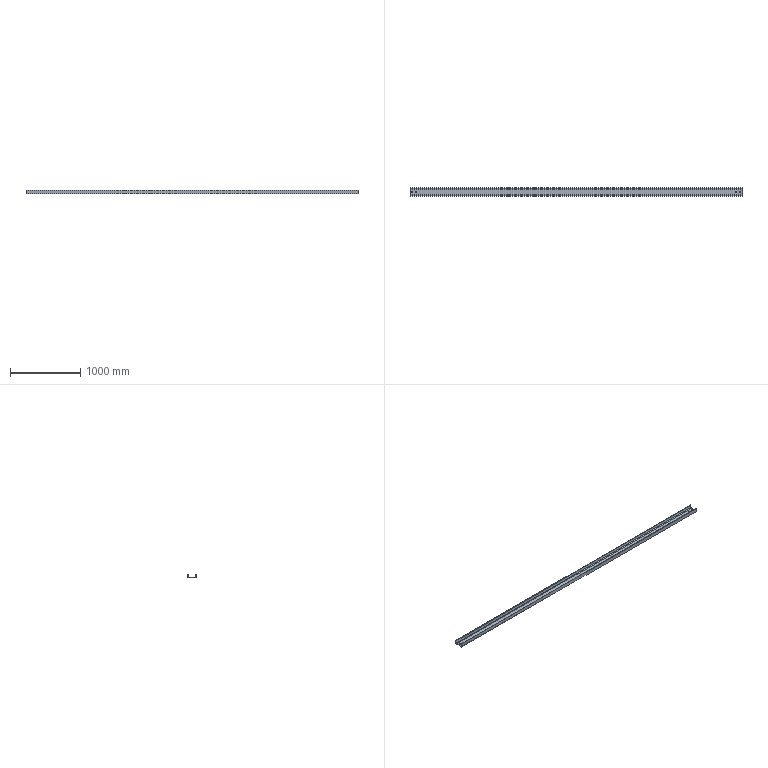Part | STEP file | E3-中转釜连接梁1_Default<As Machined> | 1 solid | 22 faces | box 4730 x 120 x 53 mm | volume 7255897 mm3 | cylinder 12 | plane 10 | commonest cylinder face diameters 19 x8 9 x2 18 x2